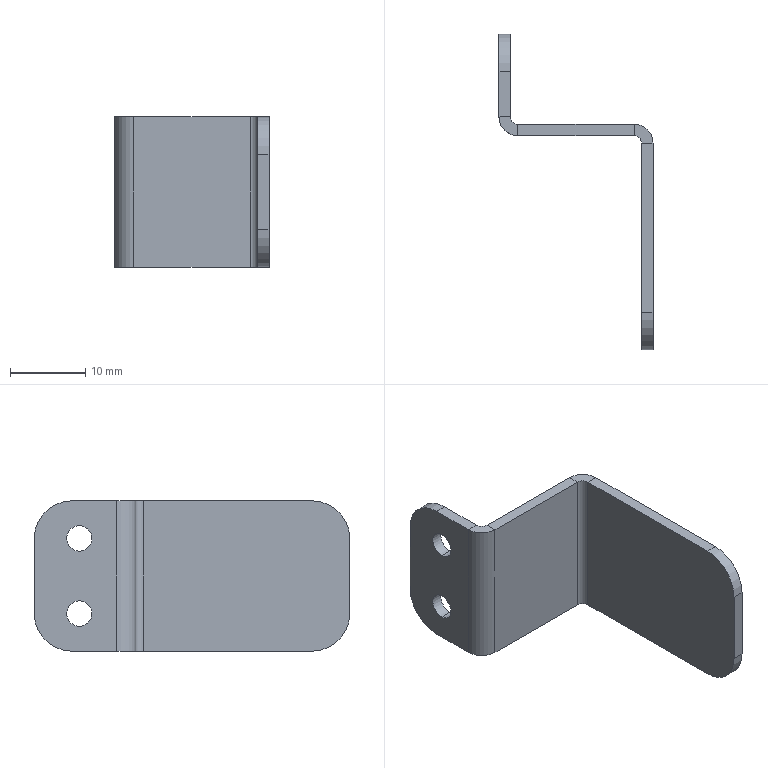Part | SolidWorks | features BreakCorner 1, FlatPattern 1, HoleWzd 1, SMBaseFlange 1, SheetMetal 1 | 1 solid | 30 faces | box 20.5 x 42 x 20 mm | volume 1726 mm3 | plane 18 | cylinder 12 | commonest cylinder face diameters 3.4 x4 10 x4 2 x2 5 x2
STEP:
#1=CARTESIAN_POINT('',(-1.5,-6.,6.7));
#2=VERTEX_POINT('',#1);
#3=CARTESIAN_POINT('',(-1.5,-6.,3.3));
#4=VERTEX_POINT('',#3);
#5=CARTESIAN_POINT('',(-1.5,-6.,5.));
#6=DIRECTION('',(1.,0.,0.));
#7=DIRECTION('',(0.,1.,0.));
#8=AXIS2_PLACEMENT_3D('',#5,#6,#7);
#9=CIRCLE('',#8,1.7);
#10=EDGE_CURVE('',#2,#4,#9,.T.);
#11=ORIENTED_EDGE('',*,*,#10,.F.);
#12=CARTESIAN_POINT('',(0.,-6.,6.7));
#13=VERTEX_POINT('',#12);
#14=CARTESIAN_POINT('',(0.,-6.,6.7));
#15=DIRECTION('',(1.,0.,0.));
#16=VECTOR('',#15,1000.);
#17=LINE('',#14,#16);
#18=EDGE_CURVE('',#2,#13,#17,.T.);
#19=ORIENTED_EDGE('',*,*,#18,.T.);
#20=CARTESIAN_POINT('',(0.,-6.,3.3));
#21=VERTEX_POINT('',#20);
#22=CARTESIAN_POINT('',(0.,-6.,5.));
#23=DIRECTION('',(1.,0.,0.));
#24=DIRECTION('',(0.,0.,-1.));
#25=AXIS2_PLACEMENT_3D('',#22,#23,#24);
#26=CIRCLE('',#25,1.7);
#27=EDGE_CURVE('',#13,#21,#26,.T.);
#28=ORIENTED_EDGE('',*,*,#27,.T.);
#29=CARTESIAN_POINT('',(0.,-6.,3.3));
#30=DIRECTION('',(1.,0.,0.));
#31=VECTOR('',#30,1000.);
#32=LINE('',#29,#31);
#33=EDGE_CURVE('',#4,#21,#32,.T.);
#34=ORIENTED_EDGE('',*,*,#33,.F.);
#35=EDGE_LOOP('',(#11,#19,#28,#34));
#36=FACE_OUTER_BOUND('',#35,.T.);
#37=CARTESIAN_POINT('',(0.,-6.,5.));
#38=DIRECTION('',(1.,0.,0.));
#39=DIRECTION('',(0.,0.,-1.));
#40=AXIS2_PLACEMENT_3D('',#37,#38,#39);
#41=CYLINDRICAL_SURFACE('',#40,1.7);
#42=ADVANCED_FACE('',(#36),#41,.F.);
#43=CARTESIAN_POINT('',(-1.5,-6.,-3.3));
#44=VERTEX_POINT('',#43);
#45=CARTESIAN_POINT('',(-1.5,-6.,-6.7));
#46=VERTEX_POINT('',#45);
#47=CARTESIAN_POINT('',(-1.5,-6.,-5.));
#48=DIRECTION('',(1.,0.,0.));
#49=DIRECTION('',(0.,1.,0.));
#50=AXIS2_PLACEMENT_3D('',#47,#48,#49);
#51=CIRCLE('',#50,1.7);
#52=EDGE_CURVE('',#44,#46,#51,.T.);
#53=ORIENTED_EDGE('',*,*,#52,.F.);
#54=CARTESIAN_POINT('',(0.,-6.,-3.3));
#55=VERTEX_POINT('',#54);
#56=CARTESIAN_POINT('',(0.,-6.,-3.3));
#57=DIRECTION('',(1.,0.,0.));
#58=VECTOR('',#57,1000.);
#59=LINE('',#56,#58);
#60=EDGE_CURVE('',#44,#55,#59,.T.);
#61=ORIENTED_EDGE('',*,*,#60,.T.);
#62=CARTESIAN_POINT('',(0.,-6.,-6.7));
#63=VERTEX_POINT('',#62);
#64=CARTESIAN_POINT('',(0.,-6.,-5.));
#65=DIRECTION('',(1.,0.,0.));
#66=DIRECTION('',(0.,0.,-1.));
#67=AXIS2_PLACEMENT_3D('',#64,#65,#66);
#68=CIRCLE('',#67,1.7);
#69=EDGE_CURVE('',#55,#63,#68,.T.);
#70=ORIENTED_EDGE('',*,*,#69,.T.);
#71=CARTESIAN_POINT('',(0.,-6.,-6.7));
#72=DIRECTION('',(1.,0.,0.));
#73=VECTOR('',#72,1000.);
#74=LINE('',#71,#73);
#75=EDGE_CURVE('',#46,#63,#74,.T.);
#76=ORIENTED_EDGE('',*,*,#75,.F.);
#77=EDGE_LOOP('',(#53,#61,#70,#76));
#78=FACE_OUTER_BOUND('',#77,.T.);
#79=CARTESIAN_POINT('',(0.,-6.,-5.));
#80=DIRECTION('',(1.,0.,0.));
#81=DIRECTION('',(0.,0.,-1.));
#82=AXIS2_PLACEMENT_3D('',#79,#80,#81);
#83=CYLINDRICAL_SURFACE('',#82,1.7);
#84=ADVANCED_FACE('',(#78),#83,.F.);
#85=CARTESIAN_POINT('',(1.,-12.,10.));
#86=VERTEX_POINT('',#85);
#87=CARTESIAN_POINT('',(1.,-13.5,10.));
#88=VERTEX_POINT('',#87);
#89=CARTESIAN_POINT('',(1.,-12.,10.));
#90=DIRECTION('',(0.,-1.,0.));
#91=VECTOR('',#90,1000.);
#92=LINE('',#89,#91);
#93=EDGE_CURVE('',#86,#88,#92,.T.);
#94=ORIENTED_EDGE('',*,*,#93,.F.);
#95=CARTESIAN_POINT('',(0.,-11.,10.));
#96=VERTEX_POINT('',#95);
#97=CARTESIAN_POINT('',(1.,-11.,10.));
#98=DIRECTION('',(0.,0.,1.));
#99=DIRECTION('',(-1.,0.,0.));
#100=AXIS2_PLACEMENT_3D('',#97,#98,#99);
#101=CIRCLE('',#100,1.);
#102=EDGE_CURVE('',#96,#86,#101,.T.);
#103=ORIENTED_EDGE('',*,*,#102,.F.);
#104=CARTESIAN_POINT('',(-1.5,-11.,10.));
#105=VERTEX_POINT('',#104);
#106=CARTESIAN_POINT('',(-1.5,-11.,10.));
#107=DIRECTION('',(1.,0.,0.));
#108=VECTOR('',#107,1000.);
#109=LINE('',#106,#108);
#110=EDGE_CURVE('',#105,#96,#109,.T.);
#111=ORIENTED_EDGE('',*,*,#110,.F.);
#112=CARTESIAN_POINT('',(1.,-11.,10.));
#113=DIRECTION('',(0.,0.,1.));
#114=DIRECTION('',(1.,0.,0.));
#115=AXIS2_PLACEMENT_3D('',#112,#113,#114);
#116=CIRCLE('',#115,2.5);
#117=EDGE_CURVE('',#105,#88,#116,.T.);
#118=ORIENTED_EDGE('',*,*,#117,.T.);
#119=EDGE_LOOP('',(#94,#103,#111,#118));
#120=FACE_OUTER_BOUND('',#119,.T.);
#121=CARTESIAN_POINT('',(1.,-12.,10.));
#122=DIRECTION('',(0.,0.,1.));
#123=DIRECTION('',(1.,0.,0.));
#124=AXIS2_PLACEMENT_3D('',#121,#122,#123);
#125=PLANE('',#124);
#126=ADVANCED_FACE('',(#120),#125,.T.);
#127=CARTESIAN_POINT('',(16.5,-12.,10.));
#128=VERTEX_POINT('',#127);
#129=CARTESIAN_POINT('',(0.,-12.,10.));
#130=DIRECTION('',(1.,0.,0.));
#131=VECTOR('',#130,1000.);
#132=LINE('',#129,#131);
#133=EDGE_CURVE('',#86,#128,#132,.T.);
#134=ORIENTED_EDGE('',*,*,#133,.F.);
#135=ORIENTED_EDGE('',*,*,#93,.T.);
#136=CARTESIAN_POINT('',(16.5,-13.5,10.));
#137=VERTEX_POINT('',#136);
#138=CARTESIAN_POINT('',(0.,-13.5,10.));
#139=DIRECTION('',(1.,0.,0.));
#140=VECTOR('',#139,1000.);
#141=LINE('',#138,#140);
#142=EDGE_CURVE('',#88,#137,#141,.T.);
#143=ORIENTED_EDGE('',*,*,#142,.T.);
#144=CARTESIAN_POINT('',(16.5,-13.5,10.));
#145=DIRECTION('',(0.,1.,0.));
#146=VECTOR('',#145,1000.);
#147=LINE('',#144,#146);
#148=EDGE_CURVE('',#137,#128,#147,.T.);
#149=ORIENTED_EDGE('',*,*,#148,.T.);
#150=EDGE_LOOP('',(#134,#135,#143,#149));
#151=FACE_OUTER_BOUND('',#150,.T.);
#152=CARTESIAN_POINT('',(-1.5,-11.,10.));
#153=DIRECTION('',(0.,0.,1.));
#154=DIRECTION('',(1.,0.,0.));
#155=AXIS2_PLACEMENT_3D('',#152,#153,#154);
#156=PLANE('',#155);
#157=ADVANCED_FACE('',(#151),#156,.T.);
#158=CARTESIAN_POINT('',(0.,-11.,-10.));
#159=VERTEX_POINT('',#158);
#160=CARTESIAN_POINT('',(-1.5,-11.,-10.));
#161=VERTEX_POINT('',#160);
#162=CARTESIAN_POINT('',(0.,-11.,-10.));
#163=DIRECTION('',(-1.,0.,0.));
#164=VECTOR('',#163,1000.);
#165=LINE('',#162,#164);
#166=EDGE_CURVE('',#159,#161,#165,.T.);
#167=ORIENTED_EDGE('',*,*,#166,.F.);
#168=CARTESIAN_POINT('',(1.,-12.,-10.));
#169=VERTEX_POINT('',#168);
#170=CARTESIAN_POINT('',(1.,-11.,-10.));
#171=DIRECTION('',(0.,0.,1.));
#172=DIRECTION('',(-1.,0.,0.));
#173=AXIS2_PLACEMENT_3D('',#170,#171,#172);
#174=CIRCLE('',#173,1.);
#175=EDGE_CURVE('',#159,#169,#174,.T.);
#176=ORIENTED_EDGE('',*,*,#175,.T.);
#177=CARTESIAN_POINT('',(1.,-13.5,-10.));
#178=VERTEX_POINT('',#177);
#179=CARTESIAN_POINT('',(1.,-13.5,-10.));
#180=DIRECTION('',(0.,1.,0.));
#181=VECTOR('',#180,1000.);
#182=LINE('',#179,#181);
#183=EDGE_CURVE('',#178,#169,#182,.T.);
#184=ORIENTED_EDGE('',*,*,#183,.F.);
#185=CARTESIAN_POINT('',(1.,-11.,-10.));
#186=DIRECTION('',(0.,0.,1.));
#187=DIRECTION('',(1.,0.,0.));
#188=AXIS2_PLACEMENT_3D('',#185,#186,#187);
#189=CIRCLE('',#188,2.5);
#190=EDGE_CURVE('',#161,#178,#189,.T.);
#191=ORIENTED_EDGE('',*,*,#190,.F.);
#192=EDGE_LOOP('',(#167,#176,#184,#191));
#193=FACE_OUTER_BOUND('',#192,.T.);
#194=CARTESIAN_POINT('',(0.,-11.,-10.));
#195=DIRECTION('',(0.,0.,-1.));
#196=DIRECTION('',(-1.,0.,0.));
#197=AXIS2_PLACEMENT_3D('',#194,#195,#196);
#198=PLANE('',#197);
#199=ADVANCED_FACE('',(#193),#198,.T.);
#200=CARTESIAN_POINT('',(-1.5,-5.,-10.));
#201=VERTEX_POINT('',#200);
#202=CARTESIAN_POINT('',(-1.5,0.,-10.));
#203=DIRECTION('',(0.,-1.,0.));
#204=VECTOR('',#203,1000.);
#205=LINE('',#202,#204);
#206=EDGE_CURVE('',#201,#161,#205,.T.);
#207=ORIENTED_EDGE('',*,*,#206,.F.);
#208=CARTESIAN_POINT('',(0.,-5.,-10.));
#209=VERTEX_POINT('',#208);
#210=CARTESIAN_POINT('',(1.,-5.,-10.));
#211=DIRECTION('',(1.,0.,0.));
#212=VECTOR('',#211,1000.);
#213=LINE('',#210,#212);
#214=EDGE_CURVE('',#201,#209,#213,.T.);
#215=ORIENTED_EDGE('',*,*,#214,.T.);
#216=CARTESIAN_POINT('',(0.,0.,-10.));
#217=DIRECTION('',(0.,-1.,0.));
#218=VECTOR('',#217,1000.);
#219=LINE('',#216,#218);
#220=EDGE_CURVE('',#209,#159,#219,.T.);
#221=ORIENTED_EDGE('',*,*,#220,.T.);
#222=ORIENTED_EDGE('',*,*,#166,.T.);
#223=EDGE_LOOP('',(#207,#215,#221,#222));
#224=FACE_OUTER_BOUND('',#223,.T.);
#225=CARTESIAN_POINT('',(1.,-13.5,-10.));
#226=DIRECTION('',(0.,0.,-1.));
#227=DIRECTION('',(-1.,0.,0.));
#228=AXIS2_PLACEMENT_3D('',#225,#226,#227);
#229=PLANE('',#228);
#230=ADVANCED_FACE('',(#224),#229,.T.);
#231=CARTESIAN_POINT('',(19.,-14.5,10.));
#232=VERTEX_POINT('',#231);
#233=CARTESIAN_POINT('',(17.5,-14.5,10.));
#234=VERTEX_POINT('',#233);
#235=CARTESIAN_POINT('',(19.,-14.5,10.));
#236=DIRECTION('',(-1.,0.,0.));
#237=VECTOR('',#236,1000.);
#238=LINE('',#235,#237);
#239=EDGE_CURVE('',#232,#234,#238,.T.);
#240=ORIENTED_EDGE('',*,*,#239,.F.);
#241=CARTESIAN_POINT('',(16.5,-14.5,10.));
#242=DIRECTION('',(0.,0.,-1.));
#243=DIRECTION('',(1.,0.,0.));
#244=AXIS2_PLACEMENT_3D('',#241,#242,#243);
#245=CIRCLE('',#244,2.5);
#246=EDGE_CURVE('',#128,#232,#245,.T.);
#247=ORIENTED_EDGE('',*,*,#246,.F.);
#248=ORIENTED_EDGE('',*,*,#148,.F.);
#249=CARTESIAN_POINT('',(16.5,-14.5,10.));
#250=DIRECTION('',(0.,0.,-1.));
#251=DIRECTION('',(1.,0.,0.));
#252=AXIS2_PLACEMENT_3D('',#249,#250,#251);
#253=CIRCLE('',#252,1.);
#254=EDGE_CURVE('',#137,#234,#253,.T.);
#255=ORIENTED_EDGE('',*,*,#254,.T.);
#256=EDGE_LOOP('',(#240,#247,#248,#255));
#257=FACE_OUTER_BOUND('',#256,.T.);
#258=CARTESIAN_POINT('',(19.,-14.5,10.));
#259=DIRECTION('',(0.,0.,1.));
#260=DIRECTION('',(1.,0.,0.));
#261=AXIS2_PLACEMENT_3D('',#258,#259,#260);
#262=PLANE('',#261);
#263=ADVANCED_FACE('',(#257),#262,.T.);
#264=CARTESIAN_POINT('',(17.5,-37.,10.));
#265=VERTEX_POINT('',#264);
#266=CARTESIAN_POINT('',(17.5,-12.,10.));
#267=DIRECTION('',(0.,-1.,0.));
#268=VECTOR('',#267,1000.);
#269=LINE('',#266,#268);
#270=EDGE_CURVE('',#234,#265,#269,.T.);
#271=ORIENTED_EDGE('',*,*,#270,.T.);
#272=CARTESIAN_POINT('',(19.,-37.,10.));
#273=VERTEX_POINT('',#272);
#274=CARTESIAN_POINT('',(16.5,-37.,10.));
#275=DIRECTION('',(1.,0.,0.));
#276=VECTOR('',#275,1000.);
#277=LINE('',#274,#276);
#278=EDGE_CURVE('',#265,#273,#277,.T.);
#279=ORIENTED_EDGE('',*,*,#278,.T.);
#280=CARTESIAN_POINT('',(19.,-12.,10.));
#281=DIRECTION('',(0.,-1.,0.));
#282=VECTOR('',#281,1000.);
#283=LINE('',#280,#282);
#284=EDGE_CURVE('',#232,#273,#283,.T.);
#285=ORIENTED_EDGE('',*,*,#284,.F.);
#286=ORIENTED_EDGE('',*,*,#239,.T.);
#287=EDGE_LOOP('',(#271,#279,#285,#286));
#288=FACE_OUTER_BOUND('',#287,.T.);
#289=CARTESIAN_POINT('',(16.5,-13.5,10.));
#290=DIRECTION('',(0.,0.,1.));
#291=DIRECTION('',(1.,0.,0.));
#292=AXIS2_PLACEMENT_3D('',#289,#290,#291);
#293=PLANE('',#292);
#294=ADVANCED_FACE('',(#288),#293,.T.);
#295=CARTESIAN_POINT('',(16.5,-12.,-10.));
#296=VERTEX_POINT('',#295);
#297=CARTESIAN_POINT('',(16.5,-13.5,-10.));
#298=VERTEX_POINT('',#297);
#299=CARTESIAN_POINT('',(16.5,-12.,-10.));
#300=DIRECTION('',(0.,-1.,0.));
#301=VECTOR('',#300,1000.);
#302=LINE('',#299,#301);
#303=EDGE_CURVE('',#296,#298,#302,.T.);
#304=ORIENTED_EDGE('',*,*,#303,.F.);
#305=CARTESIAN_POINT('',(19.,-14.5,-10.));
#306=VERTEX_POINT('',#305);
#307=CARTESIAN_POINT('',(16.5,-14.5,-10.));
#308=DIRECTION('',(0.,0.,-1.));
#309=DIRECTION('',(1.,0.,0.));
#310=AXIS2_PLACEMENT_3D('',#307,#308,#309);
#311=CIRCLE('',#310,2.5);
#312=EDGE_CURVE('',#296,#306,#311,.T.);
#313=ORIENTED_EDGE('',*,*,#312,.T.);
#314=CARTESIAN_POINT('',(17.5,-14.5,-10.));
#315=VERTEX_POINT('',#314);
#316=CARTESIAN_POINT('',(17.5,-14.5,-10.));
#317=DIRECTION('',(1.,0.,0.));
#318=VECTOR('',#317,1000.);
#319=LINE('',#316,#318);
#320=EDGE_CURVE('',#315,#306,#319,.T.);
#321=ORIENTED_EDGE('',*,*,#320,.F.);
#322=CARTESIAN_POINT('',(16.5,-14.5,-10.));
#323=DIRECTION('',(0.,0.,-1.));
#324=DIRECTION('',(1.,0.,0.));
#325=AXIS2_PLACEMENT_3D('',#322,#323,#324);
#326=CIRCLE('',#325,1.);
#327=EDGE_CURVE('',#298,#315,#326,.T.);
#328=ORIENTED_EDGE('',*,*,#327,.F.);
#329=EDGE_LOOP('',(#304,#313,#321,#328));
#330=FACE_OUTER_BOUND('',#329,.T.);
#331=CARTESIAN_POINT('',(16.5,-12.,-10.));
#332=DIRECTION('',(0.,0.,-1.));
#333=DIRECTION('',(-1.,0.,0.));
#334=AXIS2_PLACEMENT_3D('',#331,#332,#333);
#335=PLANE('',#334);
#336=ADVANCED_FACE('',(#330),#335,.T.);
#337=CARTESIAN_POINT('',(0.,-12.,-10.));
#338=DIRECTION('',(1.,0.,0.));
#339=VECTOR('',#338,1000.);
#340=LINE('',#337,#339);
#341=EDGE_CURVE('',#169,#296,#340,.T.);
#342=ORIENTED_EDGE('',*,*,#341,.T.);
#343=ORIENTED_EDGE('',*,*,#303,.T.);
#344=CARTESIAN_POINT('',(0.,-13.5,-10.));
#345=DIRECTION('',(1.,0.,0.));
#346=VECTOR('',#345,1000.);
#347=LINE('',#344,#346);
#348=EDGE_CURVE('',#178,#298,#347,.T.);
#349=ORIENTED_EDGE('',*,*,#348,.F.);
#350=ORIENTED_EDGE('',*,*,#183,.T.);
#351=EDGE_LOOP('',(#342,#343,#349,#350));
#352=FACE_OUTER_BOUND('',#351,.T.);
#353=CARTESIAN_POINT('',(17.5,-14.5,-10.));
#354=DIRECTION('',(0.,0.,-1.));
#355=DIRECTION('',(-1.,0.,0.));
#356=AXIS2_PLACEMENT_3D('',#353,#354,#355);
#357=PLANE('',#356);
#358=ADVANCED_FACE('',(#352),#357,.T.);
#359=CARTESIAN_POINT('',(17.5,-42.,5.));
#360=VERTEX_POINT('',#359);
#361=CARTESIAN_POINT('',(17.5,-42.,-5.));
#362=VERTEX_POINT('',#361);
#363=CARTESIAN_POINT('',(17.5,-42.,10.));
#364=DIRECTION('',(0.,0.,-1.));
#365=VECTOR('',#364,1000.);
#366=LINE('',#363,#365);
#367=EDGE_CURVE('',#360,#362,#366,.T.);
#368=ORIENTED_EDGE('',*,*,#367,.F.);
#369=CARTESIAN_POINT('',(17.5,-37.,5.));
#370=DIRECTION('',(-1.,0.,0.));
#371=DIRECTION('',(0.,1.,0.));
#372=AXIS2_PLACEMENT_3D('',#369,#370,#371);
#373=CIRCLE('',#372,5.);
#374=EDGE_CURVE('',#360,#265,#373,.T.);
#375=ORIENTED_EDGE('',*,*,#374,.T.);
#376=ORIENTED_EDGE('',*,*,#270,.F.);
#377=CARTESIAN_POINT('',(17.5,-14.5,10.));
#378=DIRECTION('',(0.,0.,-1.));
#379=VECTOR('',#378,1000.);
#380=LINE('',#377,#379);
#381=EDGE_CURVE('',#234,#315,#380,.T.);
#382=ORIENTED_EDGE('',*,*,#381,.T.);
#383=CARTESIAN_POINT('',(17.5,-37.,-10.));
#384=VERTEX_POINT('',#383);
#385=CARTESIAN_POINT('',(17.5,-12.,-10.));
#386=DIRECTION('',(0.,-1.,0.));
#387=VECTOR('',#386,1000.);
#388=LINE('',#385,#387);
#389=EDGE_CURVE('',#315,#384,#388,.T.);
#390=ORIENTED_EDGE('',*,*,#389,.T.);
#391=CARTESIAN_POINT('',(17.5,-37.,-5.));
#392=DIRECTION('',(-1.,0.,0.));
#393=DIRECTION('',(0.,1.,0.));
#394=AXIS2_PLACEMENT_3D('',#391,#392,#393);
#395=CIRCLE('',#394,5.);
#396=EDGE_CURVE('',#384,#362,#395,.T.);
#397=ORIENTED_EDGE('',*,*,#396,.T.);
#398=EDGE_LOOP('',(#368,#375,#376,#382,#390,#397));
#399=FACE_OUTER_BOUND('',#398,.T.);
#400=CARTESIAN_POINT('',(17.5,-12.,10.));
#401=DIRECTION('',(1.,0.,0.));
#402=DIRECTION('',(0.,1.,0.));
#403=AXIS2_PLACEMENT_3D('',#400,#401,#402);
#404=PLANE('',#403);
#405=ADVANCED_FACE('',(#399),#404,.F.);
#406=CARTESIAN_POINT('',(19.,-42.,5.));
#407=VERTEX_POINT('',#406);
#408=CARTESIAN_POINT('',(19.,-42.,-5.));
#409=VERTEX_POINT('',#408);
#410=CARTESIAN_POINT('',(19.,-42.,10.));
#411=DIRECTION('',(0.,0.,-1.));
#412=VECTOR('',#411,1000.);
#413=LINE('',#410,#412);
#414=EDGE_CURVE('',#407,#409,#413,.T.);
#415=ORIENTED_EDGE('',*,*,#414,.F.);
#416=CARTESIAN_POINT('',(19.,-42.,5.));
#417=DIRECTION('',(-1.,0.,0.));
#418=VECTOR('',#417,1000.);
#419=LINE('',#416,#418);
#420=EDGE_CURVE('',#407,#360,#419,.T.);
#421=ORIENTED_EDGE('',*,*,#420,.T.);
#422=ORIENTED_EDGE('',*,*,#367,.T.);
#423=CARTESIAN_POINT('',(19.,-42.,-5.));
#424=DIRECTION('',(1.,0.,0.));
#425=VECTOR('',#424,1000.);
#426=LINE('',#423,#425);
#427=EDGE_CURVE('',#362,#409,#426,.T.);
#428=ORIENTED_EDGE('',*,*,#427,.T.);
#429=EDGE_LOOP('',(#415,#421,#422,#428));
#430=FACE_OUTER_BOUND('',#429,.T.);
#431=CARTESIAN_POINT('',(19.,-42.,10.));
#432=DIRECTION('',(0.,-1.,0.));
#433=DIRECTION('',(0.,0.,-1.));
#434=AXIS2_PLACEMENT_3D('',#431,#432,#433);
#435=PLANE('',#434);
#436=ADVANCED_FACE('',(#430),#435,.T.);
#437=ORIENTED_EDGE('',*,*,#284,.T.);
#438=CARTESIAN_POINT('',(19.,-37.,5.));
#439=DIRECTION('',(1.,0.,0.));
#440=DIRECTION('',(0.,1.,0.));
#441=AXIS2_PLACEMENT_3D('',#438,#439,#440);
#442=CIRCLE('',#441,5.);
#443=EDGE_CURVE('',#273,#407,#442,.T.);
#444=ORIENTED_EDGE('',*,*,#443,.T.);
#445=ORIENTED_EDGE('',*,*,#414,.T.);
#446=CARTESIAN_POINT('',(19.,-37.,-10.));
#447=VERTEX_POINT('',#446);
#448=CARTESIAN_POINT('',(19.,-37.,-5.));
#449=DIRECTION('',(1.,0.,0.));
#450=DIRECTION('',(0.,1.,0.));
#451=AXIS2_PLACEMENT_3D('',#448,#449,#450);
#452=CIRCLE('',#451,5.);
#453=EDGE_CURVE('',#409,#447,#452,.T.);
#454=ORIENTED_EDGE('',*,*,#453,.T.);
#455=CARTESIAN_POINT('',(19.,-12.,-10.));
#456=DIRECTION('',(0.,-1.,0.));
#457=VECTOR('',#456,1000.);
#458=LINE('',#455,#457);
#459=EDGE_CURVE('',#306,#447,#458,.T.);
#460=ORIENTED_EDGE('',*,*,#459,.F.);
#461=CARTESIAN_POINT('',(19.,-14.5,10.));
#462=DIRECTION('',(0.,0.,-1.));
#463=VECTOR('',#462,1000.);
#464=LINE('',#461,#463);
#465=EDGE_CURVE('',#232,#306,#464,.T.);
#466=ORIENTED_EDGE('',*,*,#465,.F.);
#467=EDGE_LOOP('',(#437,#444,#445,#454,#460,#466));
#468=FACE_OUTER_BOUND('',#467,.T.);
#469=CARTESIAN_POINT('',(19.,-12.,10.));
#470=DIRECTION('',(1.,0.,0.));
#471=DIRECTION('',(0.,1.,0.));
#472=AXIS2_PLACEMENT_3D('',#469,#470,#471);
#473=PLANE('',#472);
#474=ADVANCED_FACE('',(#468),#473,.T.);
#475=ORIENTED_EDGE('',*,*,#312,.F.);
#476=CARTESIAN_POINT('',(16.5,-12.,10.));
#477=DIRECTION('',(0.,0.,-1.));
#478=VECTOR('',#477,1000.);
#479=LINE('',#476,#478);
#480=EDGE_CURVE('',#128,#296,#479,.T.);
#481=ORIENTED_EDGE('',*,*,#480,.F.);
#482=ORIENTED_EDGE('',*,*,#246,.T.);
#483=ORIENTED_EDGE('',*,*,#465,.T.);
#484=EDGE_LOOP('',(#475,#481,#482,#483));
#485=FACE_OUTER_BOUND('',#484,.T.);
#486=CARTESIAN_POINT('',(16.5,-14.5,10.));
#487=DIRECTION('',(0.,0.,-1.));
#488=DIRECTION('',(-1.,0.,0.));
#489=AXIS2_PLACEMENT_3D('',#486,#487,#488);
#490=CYLINDRICAL_SURFACE('',#489,2.5);
#491=ADVANCED_FACE('',(#485),#490,.T.);
#492=ORIENTED_EDGE('',*,*,#341,.F.);
#493=CARTESIAN_POINT('',(1.,-12.,10.));
#494=DIRECTION('',(0.,0.,-1.));
#495=VECTOR('',#494,1000.);
#496=LINE('',#493,#495);
#497=EDGE_CURVE('',#86,#169,#496,.T.);
#498=ORIENTED_EDGE('',*,*,#497,.F.);
#499=ORIENTED_EDGE('',*,*,#133,.T.);
#500=ORIENTED_EDGE('',*,*,#480,.T.);
#501=EDGE_LOOP('',(#492,#498,#499,#500));
#502=FACE_OUTER_BOUND('',#501,.T.);
#503=CARTESIAN_POINT('',(0.,-12.,10.));
#504=DIRECTION('',(0.,1.,0.));
#505=DIRECTION('',(0.,0.,1.));
#506=AXIS2_PLACEMENT_3D('',#503,#504,#505);
#507=PLANE('',#506);
#508=ADVANCED_FACE('',(#502),#507,.T.);
#509=ORIENTED_EDGE('',*,*,#175,.F.);
#510=CARTESIAN_POINT('',(0.,-11.,10.));
#511=DIRECTION('',(0.,0.,-1.));
#512=VECTOR('',#511,1000.);
#513=LINE('',#510,#512);
#514=EDGE_CURVE('',#96,#159,#513,.T.);
#515=ORIENTED_EDGE('',*,*,#514,.F.);
#516=ORIENTED_EDGE('',*,*,#102,.T.);
#517=ORIENTED_EDGE('',*,*,#497,.T.);
#518=EDGE_LOOP('',(#509,#515,#516,#517));
#519=FACE_OUTER_BOUND('',#518,.T.);
#520=CARTESIAN_POINT('',(1.,-11.,10.));
#521=DIRECTION('',(0.,0.,-1.));
#522=DIRECTION('',(-1.,0.,0.));
#523=AXIS2_PLACEMENT_3D('',#520,#521,#522);
#524=CYLINDRICAL_SURFACE('',#523,1.);
#525=ADVANCED_FACE('',(#519),#524,.F.);
#526=CARTESIAN_POINT('',(0.,-6.,5.));
#527=DIRECTION('',(1.,0.,0.));
#528=DIRECTION('',(0.,0.,-1.));
#529=AXIS2_PLACEMENT_3D('',#526,#527,#528);
#530=CIRCLE('',#529,1.7);
#531=EDGE_CURVE('',#21,#13,#530,.T.);
#532=ORIENTED_EDGE('',*,*,#531,.F.);
#533=ORIENTED_EDGE('',*,*,#27,.F.);
#534=EDGE_LOOP('',(#532,#533));
#535=FACE_BOUND('',#534,.T.);
#536=CARTESIAN_POINT('',(0.,-6.,-5.));
#537=DIRECTION('',(1.,0.,0.));
#538=DIRECTION('',(0.,0.,-1.));
#539=AXIS2_PLACEMENT_3D('',#536,#537,#538);
#540=CIRCLE('',#539,1.7);
#541=EDGE_CURVE('',#63,#55,#540,.T.);
#542=ORIENTED_EDGE('',*,*,#541,.F.);
#543=ORIENTED_EDGE('',*,*,#69,.F.);
#544=EDGE_LOOP('',(#542,#543));
#545=FACE_BOUND('',#544,.T.);
#546=CARTESIAN_POINT('',(0.,0.,5.));
#547=VERTEX_POINT('',#546);
#548=CARTESIAN_POINT('',(0.,0.,-5.));
#549=VERTEX_POINT('',#548);
#550=CARTESIAN_POINT('',(0.,0.,10.));
#551=DIRECTION('',(0.,0.,-1.));
#552=VECTOR('',#551,1000.);
#553=LINE('',#550,#552);
#554=EDGE_CURVE('',#547,#549,#553,.T.);
#555=ORIENTED_EDGE('',*,*,#554,.F.);
#556=CARTESIAN_POINT('',(0.,-5.,10.));
#557=VERTEX_POINT('',#556);
#558=CARTESIAN_POINT('',(0.,-5.,5.));
#559=DIRECTION('',(1.,0.,0.));
#560=DIRECTION('',(0.,1.,0.));
#561=AXIS2_PLACEMENT_3D('',#558,#559,#560);
#562=CIRCLE('',#561,5.);
#563=EDGE_CURVE('',#547,#557,#562,.T.);
#564=ORIENTED_EDGE('',*,*,#563,.T.);
#565=CARTESIAN_POINT('',(0.,0.,10.));
#566=DIRECTION('',(0.,-1.,0.));
#567=VECTOR('',#566,1000.);
#568=LINE('',#565,#567);
#569=EDGE_CURVE('',#557,#96,#568,.T.);
#570=ORIENTED_EDGE('',*,*,#569,.T.);
#571=ORIENTED_EDGE('',*,*,#514,.T.);
#572=ORIENTED_EDGE('',*,*,#220,.F.);
#573=CARTESIAN_POINT('',(0.,-5.,-5.));
#574=DIRECTION('',(1.,0.,0.));
#575=DIRECTION('',(0.,1.,0.));
#576=AXIS2_PLACEMENT_3D('',#573,#574,#575);
#577=CIRCLE('',#576,5.);
#578=EDGE_CURVE('',#209,#549,#577,.T.);
#579=ORIENTED_EDGE('',*,*,#578,.T.);
#580=EDGE_LOOP('',(#555,#564,#570,#571,#572,#579));
#581=FACE_OUTER_BOUND('',#580,.T.);
#582=CARTESIAN_POINT('',(0.,0.,10.));
#583=DIRECTION('',(1.,0.,0.));
#584=DIRECTION('',(0.,1.,0.));
#585=AXIS2_PLACEMENT_3D('',#582,#583,#584);
#586=PLANE('',#585);
#587=ADVANCED_FACE('',(#535,#545,#581),#586,.T.);
#588=CARTESIAN_POINT('',(-1.5,0.,5.));
#589=VERTEX_POINT('',#588);
#590=CARTESIAN_POINT('',(-1.5,0.,-5.));
#591=VERTEX_POINT('',#590);
#592=CARTESIAN_POINT('',(-1.5,0.,10.));
#593=DIRECTION('',(0.,0.,-1.));
#594=VECTOR('',#593,1000.);
#595=LINE('',#592,#594);
#596=EDGE_CURVE('',#589,#591,#595,.T.);
#597=ORIENTED_EDGE('',*,*,#596,.F.);
#598=CARTESIAN_POINT('',(-1.5,0.,5.));
#599=DIRECTION('',(1.,0.,0.));
#600=VECTOR('',#599,1000.);
#601=LINE('',#598,#600);
#602=EDGE_CURVE('',#589,#547,#601,.T.);
#603=ORIENTED_EDGE('',*,*,#602,.T.);
#604=ORIENTED_EDGE('',*,*,#554,.T.);
#605=CARTESIAN_POINT('',(-1.5,0.,-5.));
#606=DIRECTION('',(-1.,0.,0.));
#607=VECTOR('',#606,1000.);
#608=LINE('',#605,#607);
#609=EDGE_CURVE('',#549,#591,#608,.T.);
#610=ORIENTED_EDGE('',*,*,#609,.T.);
#611=EDGE_LOOP('',(#597,#603,#604,#610));
#612=FACE_OUTER_BOUND('',#611,.T.);
#613=CARTESIAN_POINT('',(-1.5,0.,10.));
#614=DIRECTION('',(0.,1.,0.));
#615=DIRECTION('',(-1.,0.,0.));
#616=AXIS2_PLACEMENT_3D('',#613,#614,#615);
#617=PLANE('',#616);
#618=ADVANCED_FACE('',(#612),#617,.T.);
#619=CARTESIAN_POINT('',(-1.5,-6.,5.));
#620=DIRECTION('',(1.,0.,0.));
#621=DIRECTION('',(0.,1.,0.));
#622=AXIS2_PLACEMENT_3D('',#619,#620,#621);
#623=CIRCLE('',#622,1.7);
#624=EDGE_CURVE('',#4,#2,#623,.T.);
#625=ORIENTED_EDGE('',*,*,#624,.T.);
#626=ORIENTED_EDGE('',*,*,#10,.T.);
#627=EDGE_LOOP('',(#625,#626));
#628=FACE_BOUND('',#627,.T.);
#629=CARTESIAN_POINT('',(-1.5,-6.,-5.));
#630=DIRECTION('',(1.,0.,0.));
#631=DIRECTION('',(0.,1.,0.));
#632=AXIS2_PLACEMENT_3D('',#629,#630,#631);
#633=CIRCLE('',#632,1.7);
#634=EDGE_CURVE('',#46,#44,#633,.T.);
#635=ORIENTED_EDGE('',*,*,#634,.T.);
#636=ORIENTED_EDGE('',*,*,#52,.T.);
#637=EDGE_LOOP('',(#635,#636));
#638=FACE_BOUND('',#637,.T.);
#639=CARTESIAN_POINT('',(-1.5,-5.,10.));
#640=VERTEX_POINT('',#639);
#641=CARTESIAN_POINT('',(-1.5,0.,10.));
#642=DIRECTION('',(0.,-1.,0.));
#643=VECTOR('',#642,1000.);
#644=LINE('',#641,#643);
#645=EDGE_CURVE('',#640,#105,#644,.T.);
#646=ORIENTED_EDGE('',*,*,#645,.F.);
#647=CARTESIAN_POINT('',(-1.5,-5.,5.));
#648=DIRECTION('',(-1.,0.,0.));
#649=DIRECTION('',(0.,1.,0.));
#650=AXIS2_PLACEMENT_3D('',#647,#648,#649);
#651=CIRCLE('',#650,5.);
#652=EDGE_CURVE('',#640,#589,#651,.T.);
#653=ORIENTED_EDGE('',*,*,#652,.T.);
#654=ORIENTED_EDGE('',*,*,#596,.T.);
#655=CARTESIAN_POINT('',(-1.5,-5.,-5.));
#656=DIRECTION('',(-1.,0.,0.));
#657=DIRECTION('',(0.,1.,0.));
#658=AXIS2_PLACEMENT_3D('',#655,#656,#657);
#659=CIRCLE('',#658,5.);
#660=EDGE_CURVE('',#591,#201,#659,.T.);
#661=ORIENTED_EDGE('',*,*,#660,.T.);
#662=ORIENTED_EDGE('',*,*,#206,.T.);
#663=CARTESIAN_POINT('',(-1.5,-11.,10.));
#664=DIRECTION('',(0.,0.,-1.));
#665=VECTOR('',#664,1000.);
#666=LINE('',#663,#665);
#667=EDGE_CURVE('',#105,#161,#666,.T.);
#668=ORIENTED_EDGE('',*,*,#667,.F.);
#669=EDGE_LOOP('',(#646,#653,#654,#661,#662,#668));
#670=FACE_OUTER_BOUND('',#669,.T.);
#671=CARTESIAN_POINT('',(-1.5,0.,10.));
#672=DIRECTION('',(1.,0.,0.));
#673=DIRECTION('',(0.,1.,0.));
#674=AXIS2_PLACEMENT_3D('',#671,#672,#673);
#675=PLANE('',#674);
#676=ADVANCED_FACE('',(#628,#638,#670),#675,.F.);
#677=ORIENTED_EDGE('',*,*,#190,.T.);
#678=CARTESIAN_POINT('',(1.,-13.5,10.));
#679=DIRECTION('',(0.,0.,-1.));
#680=VECTOR('',#679,1000.);
#681=LINE('',#678,#680);
#682=EDGE_CURVE('',#88,#178,#681,.T.);
#683=ORIENTED_EDGE('',*,*,#682,.F.);
#684=ORIENTED_EDGE('',*,*,#117,.F.);
#685=ORIENTED_EDGE('',*,*,#667,.T.);
#686=EDGE_LOOP('',(#677,#683,#684,#685));
#687=FACE_OUTER_BOUND('',#686,.T.);
#688=CARTESIAN_POINT('',(1.,-11.,10.));
#689=DIRECTION('',(0.,0.,-1.));
#690=DIRECTION('',(-1.,0.,0.));
#691=AXIS2_PLACEMENT_3D('',#688,#689,#690);
#692=CYLINDRICAL_SURFACE('',#691,2.5);
#693=ADVANCED_FACE('',(#687),#692,.T.);
#694=ORIENTED_EDGE('',*,*,#348,.T.);
#695=CARTESIAN_POINT('',(16.5,-13.5,10.));
#696=DIRECTION('',(0.,0.,-1.));
#697=VECTOR('',#696,1000.);
#698=LINE('',#695,#697);
#699=EDGE_CURVE('',#137,#298,#698,.T.);
#700=ORIENTED_EDGE('',*,*,#699,.F.);
#701=ORIENTED_EDGE('',*,*,#142,.F.);
#702=ORIENTED_EDGE('',*,*,#682,.T.);
#703=EDGE_LOOP('',(#694,#700,#701,#702));
#704=FACE_OUTER_BOUND('',#703,.T.);
#705=CARTESIAN_POINT('',(0.,-13.5,10.));
#706=DIRECTION('',(0.,1.,0.));
#707=DIRECTION('',(0.,0.,1.));
#708=AXIS2_PLACEMENT_3D('',#705,#706,#707);
#709=PLANE('',#708);
#710=ADVANCED_FACE('',(#704),#709,.F.);
#711=ORIENTED_EDGE('',*,*,#327,.T.);
#712=ORIENTED_EDGE('',*,*,#381,.F.);
#713=ORIENTED_EDGE('',*,*,#254,.F.);
#714=ORIENTED_EDGE('',*,*,#699,.T.);
#715=EDGE_LOOP('',(#711,#712,#713,#714));
#716=FACE_OUTER_BOUND('',#715,.T.);
#717=CARTESIAN_POINT('',(16.5,-14.5,10.));
#718=DIRECTION('',(0.,0.,-1.));
#719=DIRECTION('',(-1.,0.,0.));
#720=AXIS2_PLACEMENT_3D('',#717,#718,#719);
#721=CYLINDRICAL_SURFACE('',#720,1.);
#722=ADVANCED_FACE('',(#716),#721,.F.);
#723=ORIENTED_EDGE('',*,*,#569,.F.);
#724=CARTESIAN_POINT('',(16.5,-5.,10.));
#725=DIRECTION('',(-1.,0.,0.));
#726=VECTOR('',#725,1000.);
#727=LINE('',#724,#726);
#728=EDGE_CURVE('',#557,#640,#727,.T.);
#729=ORIENTED_EDGE('',*,*,#728,.T.);
#730=ORIENTED_EDGE('',*,*,#645,.T.);
#731=ORIENTED_EDGE('',*,*,#110,.T.);
#732=EDGE_LOOP('',(#723,#729,#730,#731));
#733=FACE_OUTER_BOUND('',#732,.T.);
#734=CARTESIAN_POINT('',(16.5,-14.5,10.));
#735=DIRECTION('',(0.,0.,1.));
#736=DIRECTION('',(1.,0.,0.));
#737=AXIS2_PLACEMENT_3D('',#734,#735,#736);
#738=PLANE('',#737);
#739=ADVANCED_FACE('',(#733),#738,.T.);
#740=ORIENTED_EDGE('',*,*,#459,.T.);
#741=CARTESIAN_POINT('',(17.5,-37.,-10.));
#742=DIRECTION('',(-1.,0.,0.));
#743=VECTOR('',#742,1000.);
#744=LINE('',#741,#743);
#745=EDGE_CURVE('',#447,#384,#744,.T.);
#746=ORIENTED_EDGE('',*,*,#745,.T.);
#747=ORIENTED_EDGE('',*,*,#389,.F.);
#748=ORIENTED_EDGE('',*,*,#320,.T.);
#749=EDGE_LOOP('',(#740,#746,#747,#748));
#750=FACE_OUTER_BOUND('',#749,.T.);
#751=CARTESIAN_POINT('',(16.5,-14.5,-10.));
#752=DIRECTION('',(0.,0.,1.));
#753=DIRECTION('',(1.,0.,0.));
#754=AXIS2_PLACEMENT_3D('',#751,#752,#753);
#755=PLANE('',#754);
#756=ADVANCED_FACE('',(#750),#755,.F.);
#757=ORIENTED_EDGE('',*,*,#443,.F.);
#758=ORIENTED_EDGE('',*,*,#278,.F.);
#759=ORIENTED_EDGE('',*,*,#374,.F.);
#760=ORIENTED_EDGE('',*,*,#420,.F.);
#761=EDGE_LOOP('',(#757,#758,#759,#760));
#762=FACE_OUTER_BOUND('',#761,.T.);
#763=CARTESIAN_POINT('',(19.,-37.,5.));
#764=DIRECTION('',(-1.,0.,0.));
#765=DIRECTION('',(0.,0.,1.));
#766=AXIS2_PLACEMENT_3D('',#763,#764,#765);
#767=CYLINDRICAL_SURFACE('',#766,5.);
#768=ADVANCED_FACE('',(#762),#767,.T.);
#769=ORIENTED_EDGE('',*,*,#453,.F.);
#770=ORIENTED_EDGE('',*,*,#427,.F.);
#771=ORIENTED_EDGE('',*,*,#396,.F.);
#772=ORIENTED_EDGE('',*,*,#745,.F.);
#773=EDGE_LOOP('',(#769,#770,#771,#772));
#774=FACE_OUTER_BOUND('',#773,.T.);
#775=CARTESIAN_POINT('',(16.5,-37.,-5.));
#776=DIRECTION('',(1.,0.,0.));
#777=DIRECTION('',(0.,0.,-1.));
#778=AXIS2_PLACEMENT_3D('',#775,#776,#777);
#779=CYLINDRICAL_SURFACE('',#778,5.);
#780=ADVANCED_FACE('',(#774),#779,.T.);
#781=ORIENTED_EDGE('',*,*,#652,.F.);
#782=ORIENTED_EDGE('',*,*,#728,.F.);
#783=ORIENTED_EDGE('',*,*,#563,.F.);
#784=ORIENTED_EDGE('',*,*,#602,.F.);
#785=EDGE_LOOP('',(#781,#782,#783,#784));
#786=FACE_OUTER_BOUND('',#785,.T.);
#787=CARTESIAN_POINT('',(-1.5,-5.,5.));
#788=DIRECTION('',(1.,0.,0.));
#789=DIRECTION('',(0.,1.,0.));
#790=AXIS2_PLACEMENT_3D('',#787,#788,#789);
#791=CYLINDRICAL_SURFACE('',#790,5.);
#792=ADVANCED_FACE('',(#786),#791,.T.);
#793=ORIENTED_EDGE('',*,*,#660,.F.);
#794=ORIENTED_EDGE('',*,*,#609,.F.);
#795=ORIENTED_EDGE('',*,*,#578,.F.);
#796=ORIENTED_EDGE('',*,*,#214,.F.);
#797=EDGE_LOOP('',(#793,#794,#795,#796));
#798=FACE_OUTER_BOUND('',#797,.T.);
#799=CARTESIAN_POINT('',(1.,-5.,-5.));
#800=DIRECTION('',(1.,0.,0.));
#801=DIRECTION('',(0.,1.,0.));
#802=AXIS2_PLACEMENT_3D('',#799,#800,#801);
#803=CYLINDRICAL_SURFACE('',#802,5.);
#804=ADVANCED_FACE('',(#798),#803,.T.);
#805=ORIENTED_EDGE('',*,*,#60,.F.);
#806=ORIENTED_EDGE('',*,*,#634,.F.);
#807=ORIENTED_EDGE('',*,*,#75,.T.);
#808=ORIENTED_EDGE('',*,*,#541,.T.);
#809=EDGE_LOOP('',(#805,#806,#807,#808));
#810=FACE_OUTER_BOUND('',#809,.T.);
#811=CARTESIAN_POINT('',(0.,-6.,-5.));
#812=DIRECTION('',(1.,0.,0.));
#813=DIRECTION('',(0.,0.,-1.));
#814=AXIS2_PLACEMENT_3D('',#811,#812,#813);
#815=CYLINDRICAL_SURFACE('',#814,1.7);
#816=ADVANCED_FACE('',(#810),#815,.F.);
#817=ORIENTED_EDGE('',*,*,#18,.F.);
#818=ORIENTED_EDGE('',*,*,#624,.F.);
#819=ORIENTED_EDGE('',*,*,#33,.T.);
#820=ORIENTED_EDGE('',*,*,#531,.T.);
#821=EDGE_LOOP('',(#817,#818,#819,#820));
#822=FACE_OUTER_BOUND('',#821,.T.);
#823=CARTESIAN_POINT('',(0.,-6.,5.));
#824=DIRECTION('',(1.,0.,0.));
#825=DIRECTION('',(0.,0.,-1.));
#826=AXIS2_PLACEMENT_3D('',#823,#824,#825);
#827=CYLINDRICAL_SURFACE('',#826,1.7);
#828=ADVANCED_FACE('',(#822),#827,.F.);
#829=CLOSED_SHELL('',(#42,#84,#126,#157,#199,#230,#263,#294,#336,#358,#405,#436,#474,#491,#508,#525,#587,#618,#676,#693,#710,#722,#739,#756,#768,#780,#792,#804,#816,#828));
#830=MANIFOLD_SOLID_BREP('',#829);
#831=CARTESIAN_POINT('',(0.,0.,0.));
#832=DIRECTION('',(0.,0.,1.));
#833=DIRECTION('',(1.,0.,0.));
#834=AXIS2_PLACEMENT_3D('',#831,#832,#833);
#835=(LENGTH_UNIT()NAMED_UNIT(*)SI_UNIT(.MILLI.,.METRE.));
#836=UNCERTAINTY_MEASURE_WITH_UNIT(LENGTH_MEASURE(0.00001),#835,'','');
#837=(NAMED_UNIT(*)PLANE_ANGLE_UNIT()SI_UNIT($,.RADIAN.));
#838=(NAMED_UNIT(*)SI_UNIT($,.STERADIAN.)SOLID_ANGLE_UNIT());
#839=(GEOMETRIC_REPRESENTATION_CONTEXT(3)GLOBAL_UNCERTAINTY_ASSIGNED_CONTEXT((#836))GLOBAL_UNIT_ASSIGNED_CONTEXT((#835,#837,#838))REPRESENTATION_CONTEXT('',''));
#840=ADVANCED_BREP_SHAPE_REPRESENTATION('',(#830,#834),#839);